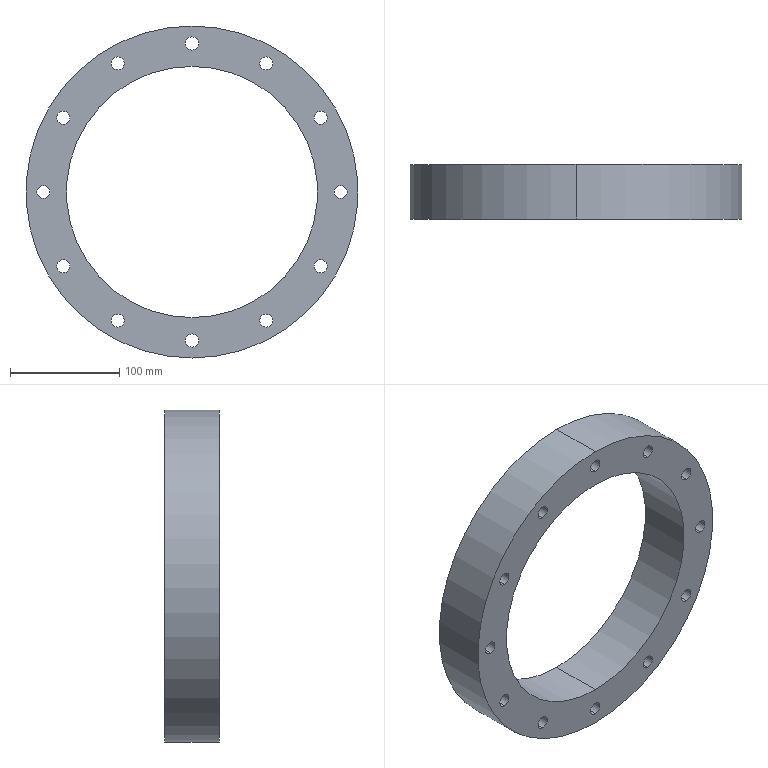Part | SolidWorks | features HoleWzd 2, ICE 2, Extrusion 1 | 1 solid | 54 faces | box 304 x 50 x 304 mm | volume 1483680 mm3 | cylinder 28 | cone 24 | plane 2 | commonest cylinder face diameters 12 x24 230 x2 304 x2